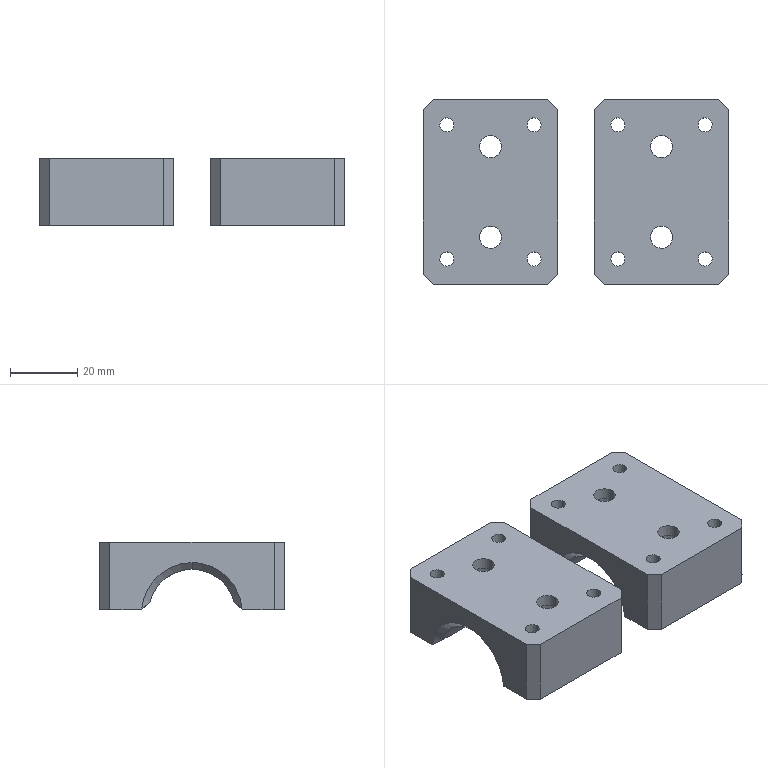NC program | NX | posted with a generic post | part box 91 x 55 x 20 mm
Lines 3974 to 4305 of 95737:
(ZLEVEL_PROFILE_COPY_1_COPY_COPY_1 , TOOL : D10JING)
N7916 T14 M6
N7918 G54
N7920 G17 G0 G90 X52.309 Y26.122 S9500 M3
N7922 G43 Z30. H14
N7924 Z-19.
N7926 G94 G1 Z-20. F1000.
N7928 X51. Y25.366
N7930 G3 X50.5 Y24.5 R1.
N7932 G1 Y-24.5 F1200.
N7934 G2 X49.036 Y-28.036 R5.
N7936 G1 X46.036 Y-31.036
N7938 G2 X42.5 Y-32.5 R5.
N7940 G1 X8.5
N7942 G2 X4.964 Y-31.036 R5.
N7944 G1 X1.964 Y-28.036
N7946 G2 X0.5 Y-24.5 R5.
N7948 G1 Y24.5
N7950 G2 X1.964 Y28.036 R5.
N7952 G1 X4.964 Y31.036
N7954 G2 X8.5 Y32.5 R5.
N7956 G1 X42.5
N7958 G2 X46.036 Y31.036 R5.
N7960 G1 X49.036 Y28.036
N7962 G2 X50.5 Y24.5 R5.
N7964 G3 X51. Y23.634 R1.
N7966 G1 X52.5 Y22.768
N7968 Z-19.
N7970 G0 Z53.
N7972 X-52.309 Y-26.122
N7974 Z-19.
N7976 G1 Z-20. F1000.
N7978 X-51. Y-25.366
N7980 G3 X-50.5 Y-24.5 R1.
N7982 G1 Y24.5 F1200.
N7984 G2 X-49.036 Y28.036 R5.
N7986 G1 X-46.036 Y31.036
N7988 G2 X-42.5 Y32.5 R5.
N7990 G1 X-8.5
N7992 G2 X-4.964 Y31.036 R5.
N7994 G1 X-1.964 Y28.036
N7996 G2 X-0.5 Y24.5 R5.
N7998 G1 Y-24.5
N8000 G2 X-1.964 Y-28.036 R5.
N8002 G1 X-4.964 Y-31.036
N8004 G2 X-8.5 Y-32.5 R5.
N8006 G1 X-42.5
N8008 G2 X-46.036 Y-31.036 R5.
N8010 G1 X-49.036 Y-28.036
N8012 G2 X-50.5 Y-24.5 R5.
N8014 G3 X-51. Y-23.634 R1.
N8016 G1 X-52.5 Y-22.768
N8018 Z-19.
N8020 G0 Z30.
N8022 M5
(HOLE_MILLING , TOOL : D6)
N8024 T12 M6
N8026 G54
N8028 G17 G0 G90 X-25.5 Y13.5 S9500 M3
N8030 G43 Z30. H12
N8032 Z0.5
N8034 G94 G3 X-26.75 Y14.75 R1.25 F1400.
N8036 X-28. Y13.5 R1.25
N8038 X-28. Y13.5 Z0. I2.5 J0.
N8040 X-28. Y13.5 Z-0.5 I2.5 J0.
N8042 X-28. Y13.5 Z-1. I2.5 J0.
N8044 X-28. Y13.5 Z-1.5 I2.5 J0.
N8046 X-28. Y13.5 Z-2. I2.5 J0.
N8048 X-28. Y13.5 Z-2.5 I2.5 J0.
N8050 X-28. Y13.5 Z-3. I2.5 J0.
N8052 X-28. Y13.5 Z-3.5 I2.5 J0.
N8054 X-28. Y13.5 Z-4. I2.5 J0.
N8056 X-28. Y13.5 Z-4.5 I2.5 J0.
N8058 X-28. Y13.5 Z-5. I2.5 J0.
N8060 X-28. Y13.5 Z-5.5 I2.5 J0.
N8062 X-28. Y13.5 Z-6. I2.5 J0.
N8064 X-28. Y13.5 Z-6.5 I2.5 J0.
N8066 X-28. Y13.5 Z-7. I2.5 J0.
N8068 X-28. Y13.5 Z-7.5 I2.5 J0.
N8070 X-28. Y13.5 Z-8. I2.5 J0.
N8072 X-28. Y13.5 Z-8.5 I2.5 J0.
N8074 X-28. Y13.5 Z-9. I2.5 J0.
N8076 X-28. Y13.5 Z-9.5 I2.5 J0.
N8078 X-28. Y13.5 Z-10. I2.5 J0.
N8080 X-28. Y13.5 Z-10.5 I2.5 J0.
N8082 X-28. Y13.5 Z-11. I2.5 J0.
N8084 X-28. Y13.5 Z-11.5 I2.5 J0.
N8086 X-28. Y13.5 Z-12. I2.5 J0.
N8088 X-28. Y13.5 Z-12.5 I2.5 J0.
N8090 X-28. Y13.5 Z-13. I2.5 J0.
N8092 X-28. Y13.5 Z-13.5 I2.5 J0.
N8094 X-28. Y13.5 Z-14. I2.5 J0.
N8096 X-28. Y13.5 Z-14.5 I2.5 J0.
N8098 X-28. Y13.5 Z-15. I2.5 J0.
N8100 X-28. Y13.5 Z-15.5 I2.5 J0.
N8102 X-28. Y13.5 Z-16. I2.5 J0.
N8104 X-28. Y13.5 Z-16.5 I2.5 J0.
N8106 X-25.5 Y11. R2.5
N8108 X-28. Y13.5 R-2.5
N8110 X-26.75 Y12.25 R1.25
N8112 X-25.5 Y13.5 R1.25
N8114 G0 Z30.
N8116 Y-13.5
N8118 Z0.5
N8120 G3 X-26.75 Y-12.25 R1.25
N8122 X-28. Y-13.5 R1.25
N8124 X-28. Y-13.5 Z0. I2.5 J0.
N8126 X-28. Y-13.5 Z-0.5 I2.5 J0.
N8128 X-28. Y-13.5 Z-1. I2.5 J0.
N8130 X-28. Y-13.5 Z-1.5 I2.5 J0.
N8132 X-28. Y-13.5 Z-2. I2.5 J0.
N8134 X-28. Y-13.5 Z-2.5 I2.5 J0.
N8136 X-28. Y-13.5 Z-3. I2.5 J0.
N8138 X-28. Y-13.5 Z-3.5 I2.5 J0.
N8140 X-28. Y-13.5 Z-4. I2.5 J0.
N8142 X-28. Y-13.5 Z-4.5 I2.5 J0.
N8144 X-28. Y-13.5 Z-5. I2.5 J0.
N8146 X-28. Y-13.5 Z-5.5 I2.5 J0.
N8148 X-28. Y-13.5 Z-6. I2.5 J0.
N8150 X-28. Y-13.5 Z-6.5 I2.5 J0.
N8152 X-28. Y-13.5 Z-7. I2.5 J0.
N8154 X-28. Y-13.5 Z-7.5 I2.5 J0.
N8156 X-28. Y-13.5 Z-8. I2.5 J0.
N8158 X-28. Y-13.5 Z-8.5 I2.5 J0.
N8160 X-28. Y-13.5 Z-9. I2.5 J0.
N8162 X-28. Y-13.5 Z-9.5 I2.5 J0.
N8164 X-28. Y-13.5 Z-10. I2.5 J0.
N8166 X-28. Y-13.5 Z-10.5 I2.5 J0.
N8168 X-28. Y-13.5 Z-11. I2.5 J0.
N8170 X-28. Y-13.5 Z-11.5 I2.5 J0.
N8172 X-28. Y-13.5 Z-12. I2.5 J0.
N8174 X-28. Y-13.5 Z-12.5 I2.5 J0.
N8176 X-28. Y-13.5 Z-13. I2.5 J0.
N8178 X-28. Y-13.5 Z-13.5 I2.5 J0.
N8180 X-28. Y-13.5 Z-14. I2.5 J0.
N8182 X-28. Y-13.5 Z-14.5 I2.5 J0.
N8184 X-28. Y-13.5 Z-15. I2.5 J0.
N8186 X-28. Y-13.5 Z-15.5 I2.5 J0.
N8188 X-28. Y-13.5 Z-16. I2.5 J0.
N8190 X-28. Y-13.5 Z-16.5 I2.5 J0.
N8192 X-25.5 Y-16. R2.5
N8194 X-28. Y-13.5 R-2.5
N8196 X-26.75 Y-14.75 R1.25
N8198 X-25.5 Y-13.5 R1.25
N8200 G0 Z30.
N8202 X25.5
N8204 Z0.5
N8206 G3 X24.25 Y-12.25 R1.25
N8208 X23. Y-13.5 R1.25
N8210 X23. Y-13.5 Z0. I2.5 J0.
N8212 X23. Y-13.5 Z-0.5 I2.5 J0.
N8214 X23. Y-13.5 Z-1. I2.5 J0.
N8216 X23. Y-13.5 Z-1.5 I2.5 J0.
N8218 X23. Y-13.5 Z-2. I2.5 J0.
N8220 X23. Y-13.5 Z-2.5 I2.5 J0.
N8222 X23. Y-13.5 Z-3. I2.5 J0.
N8224 X23. Y-13.5 Z-3.5 I2.5 J0.
N8226 X23. Y-13.5 Z-4. I2.5 J0.
N8228 X23. Y-13.5 Z-4.5 I2.5 J0.
N8230 X23. Y-13.5 Z-5. I2.5 J0.
N8232 X23. Y-13.5 Z-5.5 I2.5 J0.
N8234 X23. Y-13.5 Z-6. I2.5 J0.
N8236 X23. Y-13.5 Z-6.5 I2.5 J0.
N8238 X23. Y-13.5 Z-7. I2.5 J0.
N8240 X23. Y-13.5 Z-7.5 I2.5 J0.
N8242 X23. Y-13.5 Z-8. I2.5 J0.
N8244 X23. Y-13.5 Z-8.5 I2.5 J0.
N8246 X23. Y-13.5 Z-9. I2.5 J0.
N8248 X23. Y-13.5 Z-9.5 I2.5 J0.
N8250 X23. Y-13.5 Z-10. I2.5 J0.
N8252 X23. Y-13.5 Z-10.5 I2.5 J0.
N8254 X23. Y-13.5 Z-11. I2.5 J0.
N8256 X23. Y-13.5 Z-11.5 I2.5 J0.
N8258 X23. Y-13.5 Z-12. I2.5 J0.
N8260 X23. Y-13.5 Z-12.5 I2.5 J0.
N8262 X23. Y-13.5 Z-13. I2.5 J0.
N8264 X23. Y-13.5 Z-13.5 I2.5 J0.
N8266 X23. Y-13.5 Z-14. I2.5 J0.
N8268 X23. Y-13.5 Z-14.5 I2.5 J0.
N8270 X23. Y-13.5 Z-15. I2.5 J0.
N8272 X23. Y-13.5 Z-15.5 I2.5 J0.
N8274 X23. Y-13.5 Z-16. I2.5 J0.
N8276 X23. Y-13.5 Z-16.5 I2.5 J0.
N8278 X25.5 Y-16. R2.5
N8280 X23. Y-13.5 R-2.5
N8282 X24.25 Y-14.75 R1.25
N8284 X25.5 Y-13.5 R1.25
N8286 G0 Z30.
N8288 Y13.5
N8290 Z0.5
N8292 G3 X24.25 Y14.75 R1.25
N8294 X23. Y13.5 R1.25
N8296 X23. Y13.5 Z0. I2.5 J0.
N8298 X23. Y13.5 Z-0.5 I2.5 J0.
N8300 X23. Y13.5 Z-1. I2.5 J0.
N8302 X23. Y13.5 Z-1.5 I2.5 J0.
N8304 X23. Y13.5 Z-2. I2.5 J0.
N8306 X23. Y13.5 Z-2.5 I2.5 J0.
N8308 X23. Y13.5 Z-3. I2.5 J0.
N8310 X23. Y13.5 Z-3.5 I2.5 J0.
N8312 X23. Y13.5 Z-4. I2.5 J0.
N8314 X23. Y13.5 Z-4.5 I2.5 J0.
N8316 X23. Y13.5 Z-5. I2.5 J0.
N8318 X23. Y13.5 Z-5.5 I2.5 J0.
N8320 X23. Y13.5 Z-6. I2.5 J0.
N8322 X23. Y13.5 Z-6.5 I2.5 J0.
N8324 X23. Y13.5 Z-7. I2.5 J0.
N8326 X23. Y13.5 Z-7.5 I2.5 J0.
N8328 X23. Y13.5 Z-8. I2.5 J0.
N8330 X23. Y13.5 Z-8.5 I2.5 J0.
N8332 X23. Y13.5 Z-9. I2.5 J0.
N8334 X23. Y13.5 Z-9.5 I2.5 J0.
N8336 X23. Y13.5 Z-10. I2.5 J0.
N8338 X23. Y13.5 Z-10.5 I2.5 J0.
N8340 X23. Y13.5 Z-11. I2.5 J0.
N8342 X23. Y13.5 Z-11.5 I2.5 J0.
N8344 X23. Y13.5 Z-12. I2.5 J0.
N8346 X23. Y13.5 Z-12.5 I2.5 J0.
N8348 X23. Y13.5 Z-13. I2.5 J0.
N8350 X23. Y13.5 Z-13.5 I2.5 J0.
N8352 X23. Y13.5 Z-14. I2.5 J0.
N8354 X23. Y13.5 Z-14.5 I2.5 J0.
N8356 X23. Y13.5 Z-15. I2.5 J0.
N8358 X23. Y13.5 Z-15.5 I2.5 J0.
N8360 X23. Y13.5 Z-16. I2.5 J0.
N8362 X23. Y13.5 Z-16.5 I2.5 J0.
N8364 X25.5 Y11. R2.5
N8366 X23. Y13.5 R-2.5
N8368 X24.25 Y12.25 R1.25
N8370 X25.5 Y13.5 R1.25
N8372 G0 Z30.
(CAVITY_MILL_COPY , TOOL : D6)
N8374 X44.887 Y-0.227
N8376 Z-10.
N8378 G1 Z-11. F700.
N8380 X44.107 Y-0.868
N8382 G2 X43.605 Y-0.003 R1.
N8384 X44.406 Y1.364 R1.56 F1500.
N8386 G3 X44.641 Y1.946 R0.5
N8388 G2 X43.5 Y1.734 R2.994
N8390 G1 X7.5
N8392 G2 X6.299 Y1.943 R2.893
N8394 G3 X6.533 Y1.36 R0.5
N8396 G2 X6.529 Y-1.362 R1.56
N8398 G3 X6.295 Y-1.947 R0.5
N8400 G2 X7.382 Y-1.734 R2.887
N8402 G1 X43.529
N8404 G2 X44.649 Y-1.951 R2.996
N8406 G3 X44.412 Y-1.365 R0.5
N8408 G2 X43.605 Y-0.003 R1.56
N8410 X44.103 Y0.865 R1.
N8412 G1 X44.885 Y0.228
N8414 Z-10.
N8416 G0 X47.362 Y-1.423 Z-10.5
N8418 G1 Z-11.5 F700.
N8420 X46.374 Y-0.916
N8422 G2 X45.832 Y-0.076 R1.
N8424 G1 X43.679 Y-0.038
N8426 X43.605 Y-0.036
N8428 X43.604 Y-0.186
N8430 G2 X45.902 Y-1.313 R2.944 F1500.
N8432 G3 X46.005 Y-0.717 R0.5
N8434 G2 X46.003 Y0.713 R1.56
N8436 G3 X45.9 Y1.306 R0.5
N8438 G2 X43.5 Y0.187 R2.952
N8440 G1 X7.341
N8442 G2 X5.094 Y1.274 R2.866
N8444 G3 X4.989 Y0.69 R0.5
N8446 G2 X4.989 Y-0.69 R1.56
N8448 G3 X5.094 Y-1.274 R0.5
N8450 G2 X7.341 Y-0.187 R2.866
N8452 G1 X43.5
N8454 X43.604 Y-0.186
N8456 G3 X44.473 Y0.309 R1.
N8458 G1 X47.032 Y0.039
N8460 Z-10.5
N8462 G0 Z30.
N8464 X-44.952 Y0.229
N8466 Z-10.
N8468 G1 Z-11. F700.
N8470 X-44.174 Y0.872
N8472 G2 X-43.669 Y0.008 R1.
N8474 X-44.456 Y-1.355 R1.56 F1500.
N8476 G3 X-44.688 Y-1.931 R0.5
N8478 G2 X-43.653 Y-1.734 R2.819
N8480 G1 X-7.5
N8482 G2 X-6.337 Y-1.946 R2.955
N8484 G3 X-6.575 Y-1.361 R0.5
N8486 G2 X-6.598 Y1.361 R1.56
N8488 G3 X-6.366 Y1.937 R0.5
N8490 G2 X-7.5 Y1.734 R2.963
N8492 G1 X-43.614
N8494 G2 X-44.705 Y1.948 R2.886
N8496 G3 X-44.47 Y1.363 R0.5
N8498 G2 X-43.669 Y0.008 R1.56
N8500 X-44.165 Y-0.861 R1.
N8502 G1 X-44.949 Y-0.226
N8504 Z-10.
N8506 G0 X-47.389 Y1.5 Z-10.5
N8508 G1 Z-11.5 F700.
N8510 X-46.317 Y0.823
N8512 G2 X-45.853 Y-0.063 R1.
N8514 G1 X-44.075 Y-0.013
N8516 G2 X-43.854 Y0.02 R3.161
N8518 G1 X-43.815 Y0.019
N8520 X-43.671 Y-0.002
N8522 X-43.692 Y-0.15
N8524 X-43.435 Y-0.187 F1500.
N8526 X-7.5
N8528 G2 X-5.1 Y-1.309 R2.94
N8530 G3 X-4.997 Y-0.714 R0.5
N8532 G2 X-4.997 Y0.715 R1.56
N8534 G3 X-5.1 Y1.309 R0.5
N8536 G2 X-7.5 Y0.187 R2.957
N8538 G1 X-43.826
N8540 G2 X-45.767 Y1.174 R2.402
N8542 G1 X-45.895 Y1.351
N8544 G3 X-46.03 Y0.724 R0.5
N8546 G2 X-46.025 Y-0.715 R1.56
N8548 G3 X-45.912 Y-1.318 R0.5
N8550 G2 X-43.837 Y-0.129 R3.011
N8552 G1 X-43.692 Y-0.15
N8554 G3 X-43.228 Y0.035 R0.5
N8556 G1 Z-10.5
N8558 G0 Z30.
N8560 M5